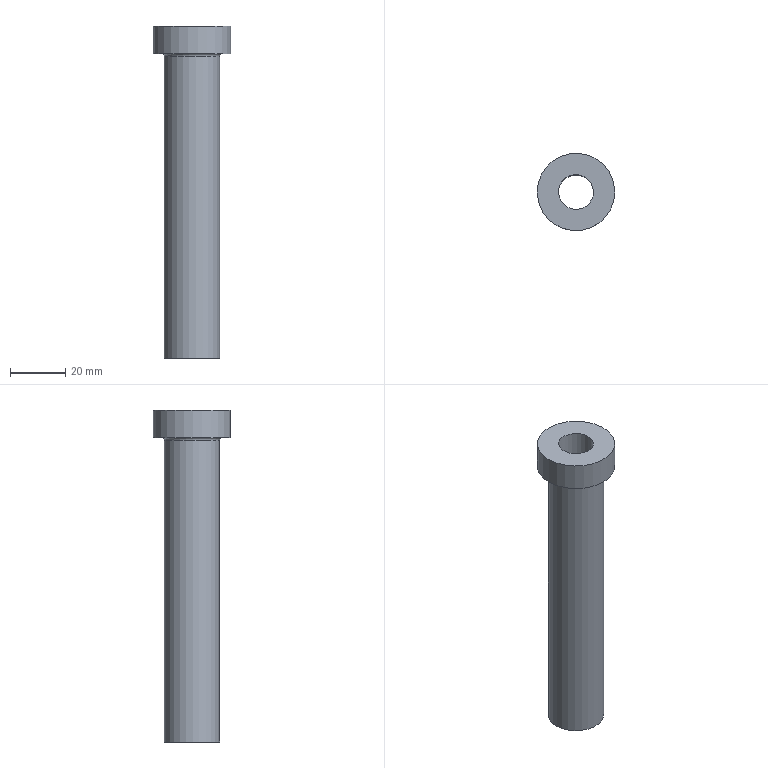Part | NX | features solid 2 | 1 solid | 7 faces | box 28 x 28 x 120 mm | volume 25766 mm3 | plane 3 | cylinder 3 | torus 1 | commonest cylinder face diameters 12.6 x1 20 x1 28 x1
STEP:
#1=CARTESIAN_POINT('',(651.479,514.689,180.));
#2=VERTEX_POINT('',#1);
#3=CARTESIAN_POINT('',(643.053,521.759,180.));
#4=DIRECTION('',(0.,0.,1.));
#5=DIRECTION('',(0.766,-0.6428,0.));
#6=AXIS2_PLACEMENT_3D('',#3,#4,#5);
#7=CIRCLE('',#6,11.);
#8=EDGE_CURVE('',#2,#2,#7,.T.);
#9=ORIENTED_EDGE('',*,*,#8,.T.);
#10=EDGE_LOOP('',(#9));
#11=FACE_BOUND('',#10,.T.);
#12=CARTESIAN_POINT('',(632.328,530.758,180.));
#13=VERTEX_POINT('',#12);
#14=CARTESIAN_POINT('',(643.053,521.759,180.));
#15=DIRECTION('',(0.,0.,-1.));
#16=DIRECTION('',(-0.766,0.6428,0.));
#17=AXIS2_PLACEMENT_3D('',#14,#15,#16);
#18=CIRCLE('',#17,14.);
#19=EDGE_CURVE('',#13,#13,#18,.T.);
#20=ORIENTED_EDGE('',*,*,#19,.T.);
#21=EDGE_LOOP('',(#20));
#22=FACE_BOUND('',#21,.T.);
#23=CARTESIAN_POINT('',(643.053,521.759,180.));
#24=DIRECTION('',(0.,0.,1.));
#25=DIRECTION('',(0.766,-0.6428,0.));
#26=AXIS2_PLACEMENT_3D('',#23,#24,#25);
#27=PLANE('',#26);
#28=ADVANCED_FACE('',(#11,#22),#27,.F.);
#29=CARTESIAN_POINT('',(647.879,517.71,190.));
#30=VERTEX_POINT('',#29);
#31=CARTESIAN_POINT('',(643.053,521.759,190.));
#32=DIRECTION('',(0.,0.,1.));
#33=DIRECTION('',(0.766,-0.6428,0.));
#34=AXIS2_PLACEMENT_3D('',#31,#32,#33);
#35=CIRCLE('',#34,6.3);
#36=EDGE_CURVE('',#30,#30,#35,.T.);
#37=ORIENTED_EDGE('',*,*,#36,.F.);
#38=EDGE_LOOP('',(#37));
#39=FACE_BOUND('',#38,.T.);
#40=CARTESIAN_POINT('',(632.328,530.758,190.));
#41=VERTEX_POINT('',#40);
#42=CARTESIAN_POINT('',(643.053,521.759,190.));
#43=DIRECTION('',(0.,0.,-1.));
#44=DIRECTION('',(-0.766,0.6428,0.));
#45=AXIS2_PLACEMENT_3D('',#42,#43,#44);
#46=CIRCLE('',#45,14.);
#47=EDGE_CURVE('',#41,#41,#46,.T.);
#48=ORIENTED_EDGE('',*,*,#47,.F.);
#49=EDGE_LOOP('',(#48));
#50=FACE_BOUND('',#49,.T.);
#51=CARTESIAN_POINT('',(643.053,521.759,190.));
#52=DIRECTION('',(0.,0.,1.));
#53=DIRECTION('',(0.766,-0.6428,0.));
#54=AXIS2_PLACEMENT_3D('',#51,#52,#53);
#55=PLANE('',#54);
#56=ADVANCED_FACE('',(#39,#50),#55,.T.);
#57=ORIENTED_EDGE('',*,*,#19,.F.);
#58=EDGE_LOOP('',(#57));
#59=FACE_BOUND('',#58,.T.);
#60=ORIENTED_EDGE('',*,*,#47,.T.);
#61=EDGE_LOOP('',(#60));
#62=FACE_BOUND('',#61,.T.);
#63=CARTESIAN_POINT('',(643.053,521.759,190.));
#64=DIRECTION('',(0.,0.,-1.));
#65=DIRECTION('',(-0.766,0.6428,0.));
#66=AXIS2_PLACEMENT_3D('',#63,#64,#65);
#67=CYLINDRICAL_SURFACE('',#66,14.);
#68=ADVANCED_FACE('',(#59,#62),#67,.T.);
#69=CARTESIAN_POINT('',(647.879,517.71,70.));
#70=VERTEX_POINT('',#69);
#71=CARTESIAN_POINT('',(643.053,521.759,70.));
#72=DIRECTION('',(0.,0.,1.));
#73=DIRECTION('',(0.766,-0.6428,0.));
#74=AXIS2_PLACEMENT_3D('',#71,#72,#73);
#75=CIRCLE('',#74,6.3);
#76=EDGE_CURVE('',#70,#70,#75,.T.);
#77=ORIENTED_EDGE('',*,*,#76,.T.);
#78=EDGE_LOOP('',(#77));
#79=FACE_BOUND('',#78,.T.);
#80=CARTESIAN_POINT('',(635.392,528.187,70.));
#81=VERTEX_POINT('',#80);
#82=CARTESIAN_POINT('',(643.053,521.759,70.));
#83=DIRECTION('',(0.,0.,-1.));
#84=DIRECTION('',(-0.766,0.6428,0.));
#85=AXIS2_PLACEMENT_3D('',#82,#83,#84);
#86=CIRCLE('',#85,10.);
#87=EDGE_CURVE('',#81,#81,#86,.T.);
#88=ORIENTED_EDGE('',*,*,#87,.T.);
#89=EDGE_LOOP('',(#88));
#90=FACE_BOUND('',#89,.T.);
#91=CARTESIAN_POINT('',(643.053,521.759,70.));
#92=DIRECTION('',(0.,0.,-1.));
#93=DIRECTION('',(-0.766,0.6428,0.));
#94=AXIS2_PLACEMENT_3D('',#91,#92,#93);
#95=PLANE('',#94);
#96=ADVANCED_FACE('',(#79,#90),#95,.T.);
#97=CARTESIAN_POINT('',(650.713,515.332,179.));
#98=VERTEX_POINT('',#97);
#99=CARTESIAN_POINT('',(643.053,521.759,179.));
#100=DIRECTION('',(0.,0.,1.));
#101=DIRECTION('',(0.766,-0.6428,0.));
#102=AXIS2_PLACEMENT_3D('',#99,#100,#101);
#103=CIRCLE('',#102,10.);
#104=EDGE_CURVE('',#98,#98,#103,.F.);
#105=ORIENTED_EDGE('',*,*,#104,.T.);
#106=EDGE_LOOP('',(#105));
#107=FACE_BOUND('',#106,.T.);
#108=ORIENTED_EDGE('',*,*,#87,.F.);
#109=EDGE_LOOP('',(#108));
#110=FACE_BOUND('',#109,.T.);
#111=CARTESIAN_POINT('',(643.053,521.759,180.));
#112=DIRECTION('',(0.,0.,-1.));
#113=DIRECTION('',(-0.766,0.6428,0.));
#114=AXIS2_PLACEMENT_3D('',#111,#112,#113);
#115=CYLINDRICAL_SURFACE('',#114,10.);
#116=ADVANCED_FACE('',(#107,#110),#115,.T.);
#117=ORIENTED_EDGE('',*,*,#36,.T.);
#118=EDGE_LOOP('',(#117));
#119=FACE_BOUND('',#118,.T.);
#120=ORIENTED_EDGE('',*,*,#76,.F.);
#121=EDGE_LOOP('',(#120));
#122=FACE_BOUND('',#121,.T.);
#123=CARTESIAN_POINT('',(643.053,521.759,70.));
#124=DIRECTION('',(0.,0.,1.));
#125=DIRECTION('',(0.766,-0.6428,0.));
#126=AXIS2_PLACEMENT_3D('',#123,#124,#125);
#127=CYLINDRICAL_SURFACE('',#126,6.3);
#128=ADVANCED_FACE('',(#119,#122),#127,.F.);
#129=ORIENTED_EDGE('',*,*,#8,.F.);
#130=EDGE_LOOP('',(#129));
#131=FACE_BOUND('',#130,.T.);
#132=ORIENTED_EDGE('',*,*,#104,.F.);
#133=EDGE_LOOP('',(#132));
#134=FACE_BOUND('',#133,.T.);
#135=CARTESIAN_POINT('',(643.053,521.759,179.));
#136=DIRECTION('',(0.,0.,1.));
#137=DIRECTION('',(0.766,-0.6428,0.));
#138=AXIS2_PLACEMENT_3D('',#135,#136,#137);
#139=TOROIDAL_SURFACE('',#138,11.,1.);
#140=ADVANCED_FACE('',(#131,#134),#139,.F.);
#141=CLOSED_SHELL('',(#28,#56,#68,#96,#116,#128,#140));
#142=MANIFOLD_SOLID_BREP('',#141);
#143=(LENGTH_UNIT()NAMED_UNIT(*)SI_UNIT(.MILLI.,.METRE.));
#144=UNCERTAINTY_MEASURE_WITH_UNIT(LENGTH_MEASURE(0.00001),#143,'','');
#145=(NAMED_UNIT(*)PLANE_ANGLE_UNIT()SI_UNIT($,.RADIAN.));
#146=(NAMED_UNIT(*)SI_UNIT($,.STERADIAN.)SOLID_ANGLE_UNIT());
#147=(GEOMETRIC_REPRESENTATION_CONTEXT(3)GLOBAL_UNCERTAINTY_ASSIGNED_CONTEXT((#144))GLOBAL_UNIT_ASSIGNED_CONTEXT((#143,#145,#146))REPRESENTATION_CONTEXT('',''));
#148=ADVANCED_BREP_SHAPE_REPRESENTATION('',(#142),#147);